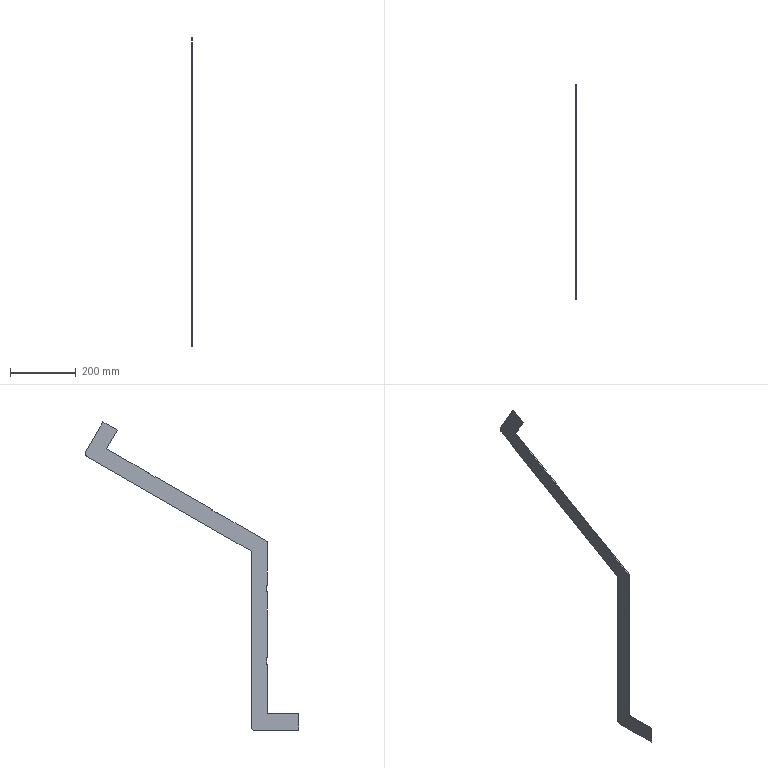Part | STEP file | zzh002 | 1 solid | 30 faces | box 3 x 648.349 x 935.758 mm | volume 197054 mm3 | plane 28 | cylinder 2 | commonest cylinder face diameters 20 x2
STEP:
#1=CARTESIAN_POINT('',(0.,380.183,431.016));
#2=VERTEX_POINT('',#1);
#3=CARTESIAN_POINT('',(0.,379.183,432.748));
#4=VERTEX_POINT('',#3);
#5=CARTESIAN_POINT('',(0.,380.183,431.016));
#6=DIRECTION('',(0.,-0.5,0.866));
#7=VECTOR('',#6,1000.);
#8=LINE('',#5,#7);
#9=EDGE_CURVE('',#2,#4,#8,.T.);
#10=ORIENTED_EDGE('',*,*,#9,.T.);
#11=CARTESIAN_POINT('',(0.,205.978,332.748));
#12=VERTEX_POINT('',#11);
#13=CARTESIAN_POINT('',(0.,379.183,432.748));
#14=DIRECTION('',(0.,-0.866,-0.5));
#15=VECTOR('',#14,1000.);
#16=LINE('',#13,#15);
#17=EDGE_CURVE('',#4,#12,#16,.T.);
#18=ORIENTED_EDGE('',*,*,#17,.T.);
#19=CARTESIAN_POINT('',(0.,206.978,331.016));
#20=VERTEX_POINT('',#19);
#21=CARTESIAN_POINT('',(0.,205.978,332.748));
#22=DIRECTION('',(0.,0.5,-0.866));
#23=VECTOR('',#22,1000.);
#24=LINE('',#21,#23);
#25=EDGE_CURVE('',#12,#20,#24,.T.);
#26=ORIENTED_EDGE('',*,*,#25,.T.);
#27=CARTESIAN_POINT('',(0.,189.658,321.016));
#28=VERTEX_POINT('',#27);
#29=CARTESIAN_POINT('',(0.,206.978,331.016));
#30=DIRECTION('',(0.,-0.866,-0.5));
#31=VECTOR('',#30,1000.);
#32=LINE('',#29,#31);
#33=EDGE_CURVE('',#20,#28,#32,.T.);
#34=ORIENTED_EDGE('',*,*,#33,.T.);
#35=CARTESIAN_POINT('',(0.,188.658,322.748));
#36=VERTEX_POINT('',#35);
#37=CARTESIAN_POINT('',(0.,189.658,321.016));
#38=DIRECTION('',(0.,-0.5,0.866));
#39=VECTOR('',#38,1000.);
#40=LINE('',#37,#39);
#41=EDGE_CURVE('',#28,#36,#40,.T.);
#42=ORIENTED_EDGE('',*,*,#41,.T.);
#43=CARTESIAN_POINT('',(0.,37.7,235.592));
#44=VERTEX_POINT('',#43);
#45=CARTESIAN_POINT('',(0.,188.658,322.748));
#46=DIRECTION('',(0.,-0.866,-0.5));
#47=VECTOR('',#46,1000.);
#48=LINE('',#45,#47);
#49=EDGE_CURVE('',#36,#44,#48,.T.);
#50=ORIENTED_EDGE('',*,*,#49,.T.);
#51=CARTESIAN_POINT('',(0.,37.7,103.281));
#52=VERTEX_POINT('',#51);
#53=CARTESIAN_POINT('',(0.,37.7,503.107));
#54=DIRECTION('',(0.,0.,-1.));
#55=VECTOR('',#54,1000.);
#56=LINE('',#53,#55);
#57=EDGE_CURVE('',#44,#52,#56,.T.);
#58=ORIENTED_EDGE('',*,*,#57,.T.);
#59=CARTESIAN_POINT('',(0.,39.7,103.281));
#60=VERTEX_POINT('',#59);
#61=CARTESIAN_POINT('',(0.,581.049,103.281));
#62=DIRECTION('',(0.,1.,0.));
#63=VECTOR('',#62,1000.);
#64=LINE('',#61,#63);
#65=EDGE_CURVE('',#52,#60,#64,.T.);
#66=ORIENTED_EDGE('',*,*,#65,.T.);
#67=CARTESIAN_POINT('',(0.,39.7,83.281));
#68=VERTEX_POINT('',#67);
#69=CARTESIAN_POINT('',(0.,39.7,503.107));
#70=DIRECTION('',(0.,0.,-1.));
#71=VECTOR('',#70,1000.);
#72=LINE('',#69,#71);
#73=EDGE_CURVE('',#60,#68,#72,.T.);
#74=ORIENTED_EDGE('',*,*,#73,.T.);
#75=CARTESIAN_POINT('',(0.,37.7,83.281));
#76=VERTEX_POINT('',#75);
#77=CARTESIAN_POINT('',(0.,581.049,83.281));
#78=DIRECTION('',(0.,-1.,0.));
#79=VECTOR('',#78,1000.);
#80=LINE('',#77,#79);
#81=EDGE_CURVE('',#68,#76,#80,.T.);
#82=ORIENTED_EDGE('',*,*,#81,.T.);
#83=CARTESIAN_POINT('',(0.,37.7,-116.719));
#84=VERTEX_POINT('',#83);
#85=CARTESIAN_POINT('',(0.,37.7,503.107));
#86=DIRECTION('',(0.,0.,-1.));
#87=VECTOR('',#86,1000.);
#88=LINE('',#85,#87);
#89=EDGE_CURVE('',#76,#84,#88,.T.);
#90=ORIENTED_EDGE('',*,*,#89,.T.);
#91=CARTESIAN_POINT('',(0.,39.7,-116.719));
#92=VERTEX_POINT('',#91);
#93=CARTESIAN_POINT('',(0.,581.049,-116.719));
#94=DIRECTION('',(0.,1.,0.));
#95=VECTOR('',#94,1000.);
#96=LINE('',#93,#95);
#97=EDGE_CURVE('',#84,#92,#96,.T.);
#98=ORIENTED_EDGE('',*,*,#97,.T.);
#99=CARTESIAN_POINT('',(0.,39.7,-136.719));
#100=VERTEX_POINT('',#99);
#101=CARTESIAN_POINT('',(0.,39.7,503.107));
#102=DIRECTION('',(0.,0.,-1.));
#103=VECTOR('',#102,1000.);
#104=LINE('',#101,#103);
#105=EDGE_CURVE('',#92,#100,#104,.T.);
#106=ORIENTED_EDGE('',*,*,#105,.T.);
#107=CARTESIAN_POINT('',(0.,37.7,-136.719));
#108=VERTEX_POINT('',#107);
#109=CARTESIAN_POINT('',(0.,581.049,-136.719));
#110=DIRECTION('',(0.,-1.,0.));
#111=VECTOR('',#110,1000.);
#112=LINE('',#109,#111);
#113=EDGE_CURVE('',#100,#108,#112,.T.);
#114=ORIENTED_EDGE('',*,*,#113,.T.);
#115=CARTESIAN_POINT('',(0.,37.7,-286.719));
#116=VERTEX_POINT('',#115);
#117=CARTESIAN_POINT('',(0.,37.7,503.107));
#118=DIRECTION('',(0.,0.,-1.));
#119=VECTOR('',#118,1000.);
#120=LINE('',#117,#119);
#121=EDGE_CURVE('',#108,#116,#120,.T.);
#122=ORIENTED_EDGE('',*,*,#121,.T.);
#123=CARTESIAN_POINT('',(0.,-57.3,-286.719));
#124=VERTEX_POINT('',#123);
#125=CARTESIAN_POINT('',(0.,581.049,-286.719));
#126=DIRECTION('',(0.,-1.,0.));
#127=VECTOR('',#126,1000.);
#128=LINE('',#125,#127);
#129=EDGE_CURVE('',#116,#124,#128,.T.);
#130=ORIENTED_EDGE('',*,*,#129,.T.);
#131=CARTESIAN_POINT('',(0.,-57.3,-336.719));
#132=VERTEX_POINT('',#131);
#133=CARTESIAN_POINT('',(0.,-57.3,503.107));
#134=DIRECTION('',(0.,0.,-1.));
#135=VECTOR('',#134,1000.);
#136=LINE('',#133,#135);
#137=EDGE_CURVE('',#124,#132,#136,.T.);
#138=ORIENTED_EDGE('',*,*,#137,.T.);
#139=CARTESIAN_POINT('',(0.,77.7,-336.719));
#140=VERTEX_POINT('',#139);
#141=CARTESIAN_POINT('',(0.,581.049,-336.719));
#142=DIRECTION('',(0.,1.,0.));
#143=VECTOR('',#142,1000.);
#144=LINE('',#141,#143);
#145=EDGE_CURVE('',#132,#140,#144,.T.);
#146=ORIENTED_EDGE('',*,*,#145,.T.);
#147=CARTESIAN_POINT('',(0.,87.7,-326.719));
#148=VERTEX_POINT('',#147);
#149=CARTESIAN_POINT('',(0.,77.7,-326.719));
#150=DIRECTION('',(1.,0.,0.));
#151=DIRECTION('',(0.,0.,-1.));
#152=AXIS2_PLACEMENT_3D('',#149,#150,#151);
#153=CIRCLE('',#152,10.);
#154=EDGE_CURVE('',#140,#148,#153,.T.);
#155=ORIENTED_EDGE('',*,*,#154,.T.);
#156=CARTESIAN_POINT('',(0.,87.7,206.725));
#157=VERTEX_POINT('',#156);
#158=CARTESIAN_POINT('',(0.,87.7,503.107));
#159=DIRECTION('',(0.,0.,1.));
#160=VECTOR('',#159,1000.);
#161=LINE('',#158,#160);
#162=EDGE_CURVE('',#148,#157,#161,.T.);
#163=ORIENTED_EDGE('',*,*,#162,.T.);
#164=CARTESIAN_POINT('',(0.,586.049,494.446));
#165=VERTEX_POINT('',#164);
#166=CARTESIAN_POINT('',(0.,87.7,206.725));
#167=DIRECTION('',(0.,0.866,0.5));
#168=VECTOR('',#167,1000.);
#169=LINE('',#166,#168);
#170=EDGE_CURVE('',#157,#165,#169,.T.);
#171=ORIENTED_EDGE('',*,*,#170,.T.);
#172=CARTESIAN_POINT('',(0.,589.709,508.107));
#173=VERTEX_POINT('',#172);
#174=CARTESIAN_POINT('',(0.,581.049,503.107));
#175=DIRECTION('',(1.,0.,0.));
#176=DIRECTION('',(0.,0.,-1.));
#177=AXIS2_PLACEMENT_3D('',#174,#175,#176);
#178=CIRCLE('',#177,10.);
#179=EDGE_CURVE('',#165,#173,#178,.T.);
#180=ORIENTED_EDGE('',*,*,#179,.T.);
#181=CARTESIAN_POINT('',(0.,537.209,599.039));
#182=VERTEX_POINT('',#181);
#183=CARTESIAN_POINT('',(0.,589.709,508.107));
#184=DIRECTION('',(0.,-0.5,0.866));
#185=VECTOR('',#184,1000.);
#186=LINE('',#183,#185);
#187=EDGE_CURVE('',#173,#182,#186,.T.);
#188=ORIENTED_EDGE('',*,*,#187,.T.);
#189=CARTESIAN_POINT('',(0.,493.908,574.039));
#190=VERTEX_POINT('',#189);
#191=CARTESIAN_POINT('',(0.,537.209,599.039));
#192=DIRECTION('',(0.,-0.866,-0.5));
#193=VECTOR('',#192,1000.);
#194=LINE('',#191,#193);
#195=EDGE_CURVE('',#182,#190,#194,.T.);
#196=ORIENTED_EDGE('',*,*,#195,.T.);
#197=CARTESIAN_POINT('',(0.,526.408,517.748));
#198=VERTEX_POINT('',#197);
#199=CARTESIAN_POINT('',(0.,493.908,574.039));
#200=DIRECTION('',(0.,0.5,-0.866));
#201=VECTOR('',#200,1000.);
#202=LINE('',#199,#201);
#203=EDGE_CURVE('',#190,#198,#202,.T.);
#204=ORIENTED_EDGE('',*,*,#203,.T.);
#205=CARTESIAN_POINT('',(0.,396.504,442.748));
#206=VERTEX_POINT('',#205);
#207=CARTESIAN_POINT('',(0.,526.408,517.748));
#208=DIRECTION('',(0.,-0.866,-0.5));
#209=VECTOR('',#208,1000.);
#210=LINE('',#207,#209);
#211=EDGE_CURVE('',#198,#206,#210,.T.);
#212=ORIENTED_EDGE('',*,*,#211,.T.);
#213=CARTESIAN_POINT('',(0.,397.504,441.016));
#214=VERTEX_POINT('',#213);
#215=CARTESIAN_POINT('',(0.,396.504,442.748));
#216=DIRECTION('',(0.,0.5,-0.866));
#217=VECTOR('',#216,1000.);
#218=LINE('',#215,#217);
#219=EDGE_CURVE('',#206,#214,#218,.T.);
#220=ORIENTED_EDGE('',*,*,#219,.T.);
#221=CARTESIAN_POINT('',(0.,397.504,441.016));
#222=DIRECTION('',(0.,-0.866,-0.5));
#223=VECTOR('',#222,1000.);
#224=LINE('',#221,#223);
#225=EDGE_CURVE('',#214,#2,#224,.T.);
#226=ORIENTED_EDGE('',*,*,#225,.T.);
#227=EDGE_LOOP('',(#10,#18,#26,#34,#42,#50,#58,#66,#74,#82,#90,#98,#106,#114,#122,#130,#138,#146,#155,#163,#171,#180,#188,#196,#204,#212,#220,#226));
#228=FACE_OUTER_BOUND('',#227,.T.);
#229=CARTESIAN_POINT('',(0.,581.049,503.107));
#230=DIRECTION('',(1.,0.,0.));
#231=DIRECTION('',(0.,0.,-1.));
#232=AXIS2_PLACEMENT_3D('',#229,#230,#231);
#233=PLANE('',#232);
#234=ADVANCED_FACE('',(#228),#233,.T.);
#235=CARTESIAN_POINT('',(-3.,379.183,432.748));
#236=VERTEX_POINT('',#235);
#237=CARTESIAN_POINT('',(-3.,379.183,432.748));
#238=DIRECTION('',(-1.,0.,0.));
#239=VECTOR('',#238,1000.);
#240=LINE('',#237,#239);
#241=EDGE_CURVE('',#4,#236,#240,.T.);
#242=ORIENTED_EDGE('',*,*,#241,.T.);
#243=CARTESIAN_POINT('',(-3.,205.978,332.748));
#244=VERTEX_POINT('',#243);
#245=CARTESIAN_POINT('',(-3.,37.7,235.592));
#246=DIRECTION('',(0.,-0.866,-0.5));
#247=VECTOR('',#246,1000.);
#248=LINE('',#245,#247);
#249=EDGE_CURVE('',#236,#244,#248,.T.);
#250=ORIENTED_EDGE('',*,*,#249,.T.);
#251=CARTESIAN_POINT('',(-3.,205.978,332.748));
#252=DIRECTION('',(1.,0.,0.));
#253=VECTOR('',#252,1000.);
#254=LINE('',#251,#253);
#255=EDGE_CURVE('',#244,#12,#254,.T.);
#256=ORIENTED_EDGE('',*,*,#255,.T.);
#257=ORIENTED_EDGE('',*,*,#17,.F.);
#258=EDGE_LOOP('',(#242,#250,#256,#257));
#259=FACE_OUTER_BOUND('',#258,.T.);
#260=CARTESIAN_POINT('',(-3.,37.7,235.592));
#261=DIRECTION('',(0.,-0.5,0.866));
#262=DIRECTION('',(0.,-0.866,-0.5));
#263=AXIS2_PLACEMENT_3D('',#260,#261,#262);
#264=PLANE('',#263);
#265=ADVANCED_FACE('',(#259),#264,.T.);
#266=ORIENTED_EDGE('',*,*,#241,.F.);
#267=ORIENTED_EDGE('',*,*,#9,.F.);
#268=CARTESIAN_POINT('',(-3.,380.183,431.016));
#269=VERTEX_POINT('',#268);
#270=CARTESIAN_POINT('',(0.,380.183,431.016));
#271=DIRECTION('',(1.,0.,0.));
#272=VECTOR('',#271,1000.);
#273=LINE('',#270,#272);
#274=EDGE_CURVE('',#269,#2,#273,.T.);
#275=ORIENTED_EDGE('',*,*,#274,.F.);
#276=CARTESIAN_POINT('',(-3.,379.183,432.748));
#277=DIRECTION('',(0.,0.5,-0.866));
#278=VECTOR('',#277,1000.);
#279=LINE('',#276,#278);
#280=EDGE_CURVE('',#236,#269,#279,.T.);
#281=ORIENTED_EDGE('',*,*,#280,.F.);
#282=EDGE_LOOP('',(#266,#267,#275,#281));
#283=FACE_OUTER_BOUND('',#282,.T.);
#284=CARTESIAN_POINT('',(0.,379.183,432.748));
#285=DIRECTION('',(0.,-0.866,-0.5));
#286=DIRECTION('',(0.,0.5,-0.866));
#287=AXIS2_PLACEMENT_3D('',#284,#285,#286);
#288=PLANE('',#287);
#289=ADVANCED_FACE('',(#283),#288,.F.);
#290=ORIENTED_EDGE('',*,*,#274,.T.);
#291=ORIENTED_EDGE('',*,*,#225,.F.);
#292=CARTESIAN_POINT('',(-3.,397.504,441.016));
#293=VERTEX_POINT('',#292);
#294=CARTESIAN_POINT('',(0.,397.504,441.016));
#295=DIRECTION('',(1.,0.,0.));
#296=VECTOR('',#295,1000.);
#297=LINE('',#294,#296);
#298=EDGE_CURVE('',#293,#214,#297,.T.);
#299=ORIENTED_EDGE('',*,*,#298,.F.);
#300=CARTESIAN_POINT('',(-3.,397.504,441.016));
#301=DIRECTION('',(0.,0.866,0.5));
#302=VECTOR('',#301,1000.);
#303=LINE('',#300,#302);
#304=EDGE_CURVE('',#269,#293,#303,.T.);
#305=ORIENTED_EDGE('',*,*,#304,.F.);
#306=EDGE_LOOP('',(#290,#291,#299,#305));
#307=FACE_OUTER_BOUND('',#306,.T.);
#308=CARTESIAN_POINT('',(0.,397.504,441.016));
#309=DIRECTION('',(0.,0.5,-0.866));
#310=DIRECTION('',(0.,0.866,0.5));
#311=AXIS2_PLACEMENT_3D('',#308,#309,#310);
#312=PLANE('',#311);
#313=ADVANCED_FACE('',(#307),#312,.F.);
#314=ORIENTED_EDGE('',*,*,#298,.T.);
#315=ORIENTED_EDGE('',*,*,#219,.F.);
#316=CARTESIAN_POINT('',(-3.,396.504,442.748));
#317=VERTEX_POINT('',#316);
#318=CARTESIAN_POINT('',(0.,396.504,442.748));
#319=DIRECTION('',(1.,0.,0.));
#320=VECTOR('',#319,1000.);
#321=LINE('',#318,#320);
#322=EDGE_CURVE('',#317,#206,#321,.T.);
#323=ORIENTED_EDGE('',*,*,#322,.F.);
#324=CARTESIAN_POINT('',(-3.,396.504,442.748));
#325=DIRECTION('',(0.,-0.5,0.866));
#326=VECTOR('',#325,1000.);
#327=LINE('',#324,#326);
#328=EDGE_CURVE('',#293,#317,#327,.T.);
#329=ORIENTED_EDGE('',*,*,#328,.F.);
#330=EDGE_LOOP('',(#314,#315,#323,#329));
#331=FACE_OUTER_BOUND('',#330,.T.);
#332=CARTESIAN_POINT('',(0.,396.504,442.748));
#333=DIRECTION('',(0.,0.866,0.5));
#334=DIRECTION('',(0.,-0.5,0.866));
#335=AXIS2_PLACEMENT_3D('',#332,#333,#334);
#336=PLANE('',#335);
#337=ADVANCED_FACE('',(#331),#336,.F.);
#338=CARTESIAN_POINT('',(-3.,526.408,517.748));
#339=VERTEX_POINT('',#338);
#340=CARTESIAN_POINT('',(-3.,526.408,517.748));
#341=DIRECTION('',(-1.,0.,0.));
#342=VECTOR('',#341,1000.);
#343=LINE('',#340,#342);
#344=EDGE_CURVE('',#198,#339,#343,.T.);
#345=ORIENTED_EDGE('',*,*,#344,.T.);
#346=CARTESIAN_POINT('',(-3.,37.7,235.592));
#347=DIRECTION('',(0.,-0.866,-0.5));
#348=VECTOR('',#347,1000.);
#349=LINE('',#346,#348);
#350=EDGE_CURVE('',#339,#317,#349,.T.);
#351=ORIENTED_EDGE('',*,*,#350,.T.);
#352=ORIENTED_EDGE('',*,*,#322,.T.);
#353=ORIENTED_EDGE('',*,*,#211,.F.);
#354=EDGE_LOOP('',(#345,#351,#352,#353));
#355=FACE_OUTER_BOUND('',#354,.T.);
#356=CARTESIAN_POINT('',(-3.,37.7,235.592));
#357=DIRECTION('',(0.,-0.5,0.866));
#358=DIRECTION('',(0.,-0.866,-0.5));
#359=AXIS2_PLACEMENT_3D('',#356,#357,#358);
#360=PLANE('',#359);
#361=ADVANCED_FACE('',(#355),#360,.T.);
#362=CARTESIAN_POINT('',(-3.,493.908,574.039));
#363=VERTEX_POINT('',#362);
#364=CARTESIAN_POINT('',(-3.,526.408,517.748));
#365=DIRECTION('',(0.,0.5,-0.866));
#366=VECTOR('',#365,1000.);
#367=LINE('',#364,#366);
#368=EDGE_CURVE('',#363,#339,#367,.T.);
#369=ORIENTED_EDGE('',*,*,#368,.T.);
#370=ORIENTED_EDGE('',*,*,#344,.F.);
#371=ORIENTED_EDGE('',*,*,#203,.F.);
#372=CARTESIAN_POINT('',(-3.,493.908,574.039));
#373=DIRECTION('',(-1.,0.,0.));
#374=VECTOR('',#373,1000.);
#375=LINE('',#372,#374);
#376=EDGE_CURVE('',#190,#363,#375,.T.);
#377=ORIENTED_EDGE('',*,*,#376,.T.);
#378=EDGE_LOOP('',(#369,#370,#371,#377));
#379=FACE_OUTER_BOUND('',#378,.T.);
#380=CARTESIAN_POINT('',(-3.,526.408,517.748));
#381=DIRECTION('',(0.,-0.866,-0.5));
#382=DIRECTION('',(0.,0.5,-0.866));
#383=AXIS2_PLACEMENT_3D('',#380,#381,#382);
#384=PLANE('',#383);
#385=ADVANCED_FACE('',(#379),#384,.T.);
#386=CARTESIAN_POINT('',(-3.,537.209,599.039));
#387=VERTEX_POINT('',#386);
#388=CARTESIAN_POINT('',(-3.,537.209,599.039));
#389=DIRECTION('',(0.,-0.866,-0.5));
#390=VECTOR('',#389,1000.);
#391=LINE('',#388,#390);
#392=EDGE_CURVE('',#387,#363,#391,.T.);
#393=ORIENTED_EDGE('',*,*,#392,.T.);
#394=ORIENTED_EDGE('',*,*,#376,.F.);
#395=ORIENTED_EDGE('',*,*,#195,.F.);
#396=CARTESIAN_POINT('',(-3.,537.209,599.039));
#397=DIRECTION('',(-1.,0.,0.));
#398=VECTOR('',#397,1000.);
#399=LINE('',#396,#398);
#400=EDGE_CURVE('',#182,#387,#399,.T.);
#401=ORIENTED_EDGE('',*,*,#400,.T.);
#402=EDGE_LOOP('',(#393,#394,#395,#401));
#403=FACE_OUTER_BOUND('',#402,.T.);
#404=CARTESIAN_POINT('',(-3.,537.209,599.039));
#405=DIRECTION('',(0.,-0.5,0.866));
#406=DIRECTION('',(0.,-0.866,-0.5));
#407=AXIS2_PLACEMENT_3D('',#404,#405,#406);
#408=PLANE('',#407);
#409=ADVANCED_FACE('',(#403),#408,.T.);
#410=CARTESIAN_POINT('',(-3.,589.709,508.107));
#411=VERTEX_POINT('',#410);
#412=CARTESIAN_POINT('',(-3.,589.709,508.107));
#413=DIRECTION('',(0.,-0.5,0.866));
#414=VECTOR('',#413,1000.);
#415=LINE('',#412,#414);
#416=EDGE_CURVE('',#411,#387,#415,.T.);
#417=ORIENTED_EDGE('',*,*,#416,.T.);
#418=ORIENTED_EDGE('',*,*,#400,.F.);
#419=ORIENTED_EDGE('',*,*,#187,.F.);
#420=CARTESIAN_POINT('',(-3.,589.709,508.107));
#421=DIRECTION('',(-1.,0.,0.));
#422=VECTOR('',#421,1000.);
#423=LINE('',#420,#422);
#424=EDGE_CURVE('',#173,#411,#423,.T.);
#425=ORIENTED_EDGE('',*,*,#424,.T.);
#426=EDGE_LOOP('',(#417,#418,#419,#425));
#427=FACE_OUTER_BOUND('',#426,.T.);
#428=CARTESIAN_POINT('',(-3.,589.709,508.107));
#429=DIRECTION('',(0.,0.866,0.5));
#430=DIRECTION('',(0.,-0.5,0.866));
#431=AXIS2_PLACEMENT_3D('',#428,#429,#430);
#432=PLANE('',#431);
#433=ADVANCED_FACE('',(#427),#432,.T.);
#434=CARTESIAN_POINT('',(-3.,586.049,494.446));
#435=VERTEX_POINT('',#434);
#436=CARTESIAN_POINT('',(-3.,581.049,503.107));
#437=DIRECTION('',(1.,0.,0.));
#438=DIRECTION('',(0.,0.,-1.));
#439=AXIS2_PLACEMENT_3D('',#436,#437,#438);
#440=CIRCLE('',#439,10.);
#441=EDGE_CURVE('',#435,#411,#440,.T.);
#442=ORIENTED_EDGE('',*,*,#441,.T.);
#443=ORIENTED_EDGE('',*,*,#424,.F.);
#444=ORIENTED_EDGE('',*,*,#179,.F.);
#445=CARTESIAN_POINT('',(-3.,586.049,494.446));
#446=DIRECTION('',(-1.,0.,0.));
#447=VECTOR('',#446,1000.);
#448=LINE('',#445,#447);
#449=EDGE_CURVE('',#165,#435,#448,.T.);
#450=ORIENTED_EDGE('',*,*,#449,.T.);
#451=EDGE_LOOP('',(#442,#443,#444,#450));
#452=FACE_OUTER_BOUND('',#451,.T.);
#453=CARTESIAN_POINT('',(-3.,581.049,503.107));
#454=DIRECTION('',(1.,0.,0.));
#455=DIRECTION('',(0.,0.,-1.));
#456=AXIS2_PLACEMENT_3D('',#453,#454,#455);
#457=CYLINDRICAL_SURFACE('',#456,10.);
#458=ADVANCED_FACE('',(#452),#457,.T.);
#459=CARTESIAN_POINT('',(-3.,87.7,206.725));
#460=VERTEX_POINT('',#459);
#461=CARTESIAN_POINT('',(-3.,87.7,206.725));
#462=DIRECTION('',(0.,0.866,0.5));
#463=VECTOR('',#462,1000.);
#464=LINE('',#461,#463);
#465=EDGE_CURVE('',#460,#435,#464,.T.);
#466=ORIENTED_EDGE('',*,*,#465,.T.);
#467=ORIENTED_EDGE('',*,*,#449,.F.);
#468=ORIENTED_EDGE('',*,*,#170,.F.);
#469=CARTESIAN_POINT('',(-3.,87.7,206.725));
#470=DIRECTION('',(-1.,0.,0.));
#471=VECTOR('',#470,1000.);
#472=LINE('',#469,#471);
#473=EDGE_CURVE('',#157,#460,#472,.T.);
#474=ORIENTED_EDGE('',*,*,#473,.T.);
#475=EDGE_LOOP('',(#466,#467,#468,#474));
#476=FACE_OUTER_BOUND('',#475,.T.);
#477=CARTESIAN_POINT('',(-3.,87.7,206.725));
#478=DIRECTION('',(0.,0.5,-0.866));
#479=DIRECTION('',(0.,0.866,0.5));
#480=AXIS2_PLACEMENT_3D('',#477,#478,#479);
#481=PLANE('',#480);
#482=ADVANCED_FACE('',(#476),#481,.T.);
#483=CARTESIAN_POINT('',(-3.,87.7,-326.719));
#484=VERTEX_POINT('',#483);
#485=CARTESIAN_POINT('',(-3.,87.7,-326.719));
#486=DIRECTION('',(0.,0.,1.));
#487=VECTOR('',#486,1000.);
#488=LINE('',#485,#487);
#489=EDGE_CURVE('',#484,#460,#488,.T.);
#490=ORIENTED_EDGE('',*,*,#489,.T.);
#491=ORIENTED_EDGE('',*,*,#473,.F.);
#492=ORIENTED_EDGE('',*,*,#162,.F.);
#493=CARTESIAN_POINT('',(-3.,87.7,-326.719));
#494=DIRECTION('',(-1.,0.,0.));
#495=VECTOR('',#494,1000.);
#496=LINE('',#493,#495);
#497=EDGE_CURVE('',#148,#484,#496,.T.);
#498=ORIENTED_EDGE('',*,*,#497,.T.);
#499=EDGE_LOOP('',(#490,#491,#492,#498));
#500=FACE_OUTER_BOUND('',#499,.T.);
#501=CARTESIAN_POINT('',(-3.,87.7,-326.719));
#502=DIRECTION('',(0.,1.,0.));
#503=DIRECTION('',(0.,0.,1.));
#504=AXIS2_PLACEMENT_3D('',#501,#502,#503);
#505=PLANE('',#504);
#506=ADVANCED_FACE('',(#500),#505,.T.);
#507=CARTESIAN_POINT('',(-3.,77.7,-336.719));
#508=VERTEX_POINT('',#507);
#509=CARTESIAN_POINT('',(-3.,77.7,-326.719));
#510=DIRECTION('',(1.,0.,0.));
#511=DIRECTION('',(0.,0.,-1.));
#512=AXIS2_PLACEMENT_3D('',#509,#510,#511);
#513=CIRCLE('',#512,10.);
#514=EDGE_CURVE('',#508,#484,#513,.T.);
#515=ORIENTED_EDGE('',*,*,#514,.T.);
#516=ORIENTED_EDGE('',*,*,#497,.F.);
#517=ORIENTED_EDGE('',*,*,#154,.F.);
#518=CARTESIAN_POINT('',(-3.,77.7,-336.719));
#519=DIRECTION('',(-1.,0.,0.));
#520=VECTOR('',#519,1000.);
#521=LINE('',#518,#520);
#522=EDGE_CURVE('',#140,#508,#521,.T.);
#523=ORIENTED_EDGE('',*,*,#522,.T.);
#524=EDGE_LOOP('',(#515,#516,#517,#523));
#525=FACE_OUTER_BOUND('',#524,.T.);
#526=CARTESIAN_POINT('',(-3.,77.7,-326.719));
#527=DIRECTION('',(1.,0.,0.));
#528=DIRECTION('',(0.,0.,-1.));
#529=AXIS2_PLACEMENT_3D('',#526,#527,#528);
#530=CYLINDRICAL_SURFACE('',#529,10.);
#531=ADVANCED_FACE('',(#525),#530,.T.);
#532=CARTESIAN_POINT('',(-3.,-57.3,-336.719));
#533=VERTEX_POINT('',#532);
#534=CARTESIAN_POINT('',(-3.,-52.5,-336.719));
#535=DIRECTION('',(0.,1.,0.));
#536=VECTOR('',#535,1000.);
#537=LINE('',#534,#536);
#538=EDGE_CURVE('',#533,#508,#537,.T.);
#539=ORIENTED_EDGE('',*,*,#538,.T.);
#540=ORIENTED_EDGE('',*,*,#522,.F.);
#541=ORIENTED_EDGE('',*,*,#145,.F.);
#542=CARTESIAN_POINT('',(-3.,-57.3,-336.719));
#543=DIRECTION('',(-1.,0.,0.));
#544=VECTOR('',#543,1000.);
#545=LINE('',#542,#544);
#546=EDGE_CURVE('',#132,#533,#545,.T.);
#547=ORIENTED_EDGE('',*,*,#546,.T.);
#548=EDGE_LOOP('',(#539,#540,#541,#547));
#549=FACE_OUTER_BOUND('',#548,.T.);
#550=CARTESIAN_POINT('',(-3.,-52.5,-336.719));
#551=DIRECTION('',(0.,0.,-1.));
#552=DIRECTION('',(0.,1.,0.));
#553=AXIS2_PLACEMENT_3D('',#550,#551,#552);
#554=PLANE('',#553);
#555=ADVANCED_FACE('',(#549),#554,.T.);
#556=CARTESIAN_POINT('',(-3.,-57.3,-286.719));
#557=VERTEX_POINT('',#556);
#558=CARTESIAN_POINT('',(-3.,-57.3,-286.719));
#559=DIRECTION('',(0.,0.,-1.));
#560=VECTOR('',#559,1000.);
#561=LINE('',#558,#560);
#562=EDGE_CURVE('',#557,#533,#561,.T.);
#563=ORIENTED_EDGE('',*,*,#562,.T.);
#564=ORIENTED_EDGE('',*,*,#546,.F.);
#565=ORIENTED_EDGE('',*,*,#137,.F.);
#566=CARTESIAN_POINT('',(-3.,-57.3,-286.719));
#567=DIRECTION('',(-1.,0.,0.));
#568=VECTOR('',#567,1000.);
#569=LINE('',#566,#568);
#570=EDGE_CURVE('',#124,#557,#569,.T.);
#571=ORIENTED_EDGE('',*,*,#570,.T.);
#572=EDGE_LOOP('',(#563,#564,#565,#571));
#573=FACE_OUTER_BOUND('',#572,.T.);
#574=CARTESIAN_POINT('',(-3.,-57.3,-286.719));
#575=DIRECTION('',(0.,-1.,0.));
#576=DIRECTION('',(0.,0.,-1.));
#577=AXIS2_PLACEMENT_3D('',#574,#575,#576);
#578=PLANE('',#577);
#579=ADVANCED_FACE('',(#573),#578,.T.);
#580=CARTESIAN_POINT('',(-3.,37.7,-286.719));
#581=VERTEX_POINT('',#580);
#582=CARTESIAN_POINT('',(-3.,-52.5,-286.719));
#583=DIRECTION('',(0.,-1.,0.));
#584=VECTOR('',#583,1000.);
#585=LINE('',#582,#584);
#586=EDGE_CURVE('',#581,#557,#585,.T.);
#587=ORIENTED_EDGE('',*,*,#586,.T.);
#588=ORIENTED_EDGE('',*,*,#570,.F.);
#589=ORIENTED_EDGE('',*,*,#129,.F.);
#590=CARTESIAN_POINT('',(-3.,37.7,-286.719));
#591=DIRECTION('',(-1.,0.,0.));
#592=VECTOR('',#591,1000.);
#593=LINE('',#590,#592);
#594=EDGE_CURVE('',#116,#581,#593,.T.);
#595=ORIENTED_EDGE('',*,*,#594,.T.);
#596=EDGE_LOOP('',(#587,#588,#589,#595));
#597=FACE_OUTER_BOUND('',#596,.T.);
#598=CARTESIAN_POINT('',(-3.,-52.5,-286.719));
#599=DIRECTION('',(0.,0.,1.));
#600=DIRECTION('',(1.,0.,0.));
#601=AXIS2_PLACEMENT_3D('',#598,#599,#600);
#602=PLANE('',#601);
#603=ADVANCED_FACE('',(#597),#602,.T.);
#604=ORIENTED_EDGE('',*,*,#594,.F.);
#605=ORIENTED_EDGE('',*,*,#121,.F.);
#606=CARTESIAN_POINT('',(-3.,37.7,-136.719));
#607=VERTEX_POINT('',#606);
#608=CARTESIAN_POINT('',(-3.,37.7,-136.719));
#609=DIRECTION('',(-1.,0.,0.));
#610=VECTOR('',#609,1000.);
#611=LINE('',#608,#610);
#612=EDGE_CURVE('',#108,#607,#611,.T.);
#613=ORIENTED_EDGE('',*,*,#612,.T.);
#614=CARTESIAN_POINT('',(-3.,37.7,-286.719));
#615=DIRECTION('',(0.,0.,-1.));
#616=VECTOR('',#615,1000.);
#617=LINE('',#614,#616);
#618=EDGE_CURVE('',#607,#581,#617,.T.);
#619=ORIENTED_EDGE('',*,*,#618,.T.);
#620=EDGE_LOOP('',(#604,#605,#613,#619));
#621=FACE_OUTER_BOUND('',#620,.T.);
#622=CARTESIAN_POINT('',(-3.,37.7,-286.719));
#623=DIRECTION('',(0.,-1.,0.));
#624=DIRECTION('',(0.,0.,-1.));
#625=AXIS2_PLACEMENT_3D('',#622,#623,#624);
#626=PLANE('',#625);
#627=ADVANCED_FACE('',(#621),#626,.T.);
#628=ORIENTED_EDGE('',*,*,#612,.F.);
#629=ORIENTED_EDGE('',*,*,#113,.F.);
#630=CARTESIAN_POINT('',(-3.,39.7,-136.719));
#631=VERTEX_POINT('',#630);
#632=CARTESIAN_POINT('',(0.,39.7,-136.719));
#633=DIRECTION('',(1.,0.,0.));
#634=VECTOR('',#633,1000.);
#635=LINE('',#632,#634);
#636=EDGE_CURVE('',#631,#100,#635,.T.);
#637=ORIENTED_EDGE('',*,*,#636,.F.);
#638=CARTESIAN_POINT('',(-3.,37.7,-136.719));
#639=DIRECTION('',(0.,1.,0.));
#640=VECTOR('',#639,1000.);
#641=LINE('',#638,#640);
#642=EDGE_CURVE('',#607,#631,#641,.T.);
#643=ORIENTED_EDGE('',*,*,#642,.F.);
#644=EDGE_LOOP('',(#628,#629,#637,#643));
#645=FACE_OUTER_BOUND('',#644,.T.);
#646=CARTESIAN_POINT('',(0.,37.7,-136.719));
#647=DIRECTION('',(0.,0.,-1.));
#648=DIRECTION('',(-1.,0.,0.));
#649=AXIS2_PLACEMENT_3D('',#646,#647,#648);
#650=PLANE('',#649);
#651=ADVANCED_FACE('',(#645),#650,.F.);
#652=ORIENTED_EDGE('',*,*,#636,.T.);
#653=ORIENTED_EDGE('',*,*,#105,.F.);
#654=CARTESIAN_POINT('',(-3.,39.7,-116.719));
#655=VERTEX_POINT('',#654);
#656=CARTESIAN_POINT('',(0.,39.7,-116.719));
#657=DIRECTION('',(1.,0.,0.));
#658=VECTOR('',#657,1000.);
#659=LINE('',#656,#658);
#660=EDGE_CURVE('',#655,#92,#659,.T.);
#661=ORIENTED_EDGE('',*,*,#660,.F.);
#662=CARTESIAN_POINT('',(-3.,39.7,-136.719));
#663=DIRECTION('',(0.,0.,1.));
#664=VECTOR('',#663,1000.);
#665=LINE('',#662,#664);
#666=EDGE_CURVE('',#631,#655,#665,.T.);
#667=ORIENTED_EDGE('',*,*,#666,.F.);
#668=EDGE_LOOP('',(#652,#653,#661,#667));
#669=FACE_OUTER_BOUND('',#668,.T.);
#670=CARTESIAN_POINT('',(0.,39.7,-136.719));
#671=DIRECTION('',(0.,1.,0.));
#672=DIRECTION('',(0.,0.,1.));
#673=AXIS2_PLACEMENT_3D('',#670,#671,#672);
#674=PLANE('',#673);
#675=ADVANCED_FACE('',(#669),#674,.F.);
#676=ORIENTED_EDGE('',*,*,#660,.T.);
#677=ORIENTED_EDGE('',*,*,#97,.F.);
#678=CARTESIAN_POINT('',(-3.,37.7,-116.719));
#679=VERTEX_POINT('',#678);
#680=CARTESIAN_POINT('',(0.,37.7,-116.719));
#681=DIRECTION('',(1.,0.,0.));
#682=VECTOR('',#681,1000.);
#683=LINE('',#680,#682);
#684=EDGE_CURVE('',#679,#84,#683,.T.);
#685=ORIENTED_EDGE('',*,*,#684,.F.);
#686=CARTESIAN_POINT('',(-3.,37.7,-116.719));
#687=DIRECTION('',(0.,-1.,0.));
#688=VECTOR('',#687,1000.);
#689=LINE('',#686,#688);
#690=EDGE_CURVE('',#655,#679,#689,.T.);
#691=ORIENTED_EDGE('',*,*,#690,.F.);
#692=EDGE_LOOP('',(#676,#677,#685,#691));
#693=FACE_OUTER_BOUND('',#692,.T.);
#694=CARTESIAN_POINT('',(0.,37.7,-116.719));
#695=DIRECTION('',(0.,0.,1.));
#696=DIRECTION('',(1.,0.,0.));
#697=AXIS2_PLACEMENT_3D('',#694,#695,#696);
#698=PLANE('',#697);
#699=ADVANCED_FACE('',(#693),#698,.F.);
#700=ORIENTED_EDGE('',*,*,#684,.T.);
#701=ORIENTED_EDGE('',*,*,#89,.F.);
#702=CARTESIAN_POINT('',(-3.,37.7,83.281));
#703=VERTEX_POINT('',#702);
#704=CARTESIAN_POINT('',(-3.,37.7,83.281));
#705=DIRECTION('',(-1.,0.,0.));
#706=VECTOR('',#705,1000.);
#707=LINE('',#704,#706);
#708=EDGE_CURVE('',#76,#703,#707,.T.);
#709=ORIENTED_EDGE('',*,*,#708,.T.);
#710=CARTESIAN_POINT('',(-3.,37.7,-286.719));
#711=DIRECTION('',(0.,0.,-1.));
#712=VECTOR('',#711,1000.);
#713=LINE('',#710,#712);
#714=EDGE_CURVE('',#703,#679,#713,.T.);
#715=ORIENTED_EDGE('',*,*,#714,.T.);
#716=EDGE_LOOP('',(#700,#701,#709,#715));
#717=FACE_OUTER_BOUND('',#716,.T.);
#718=CARTESIAN_POINT('',(-3.,37.7,-286.719));
#719=DIRECTION('',(0.,-1.,0.));
#720=DIRECTION('',(0.,0.,-1.));
#721=AXIS2_PLACEMENT_3D('',#718,#719,#720);
#722=PLANE('',#721);
#723=ADVANCED_FACE('',(#717),#722,.T.);
#724=ORIENTED_EDGE('',*,*,#708,.F.);
#725=ORIENTED_EDGE('',*,*,#81,.F.);
#726=CARTESIAN_POINT('',(-3.,39.7,83.281));
#727=VERTEX_POINT('',#726);
#728=CARTESIAN_POINT('',(0.,39.7,83.281));
#729=DIRECTION('',(1.,0.,0.));
#730=VECTOR('',#729,1000.);
#731=LINE('',#728,#730);
#732=EDGE_CURVE('',#727,#68,#731,.T.);
#733=ORIENTED_EDGE('',*,*,#732,.F.);
#734=CARTESIAN_POINT('',(-3.,37.7,83.281));
#735=DIRECTION('',(0.,1.,0.));
#736=VECTOR('',#735,1000.);
#737=LINE('',#734,#736);
#738=EDGE_CURVE('',#703,#727,#737,.T.);
#739=ORIENTED_EDGE('',*,*,#738,.F.);
#740=EDGE_LOOP('',(#724,#725,#733,#739));
#741=FACE_OUTER_BOUND('',#740,.T.);
#742=CARTESIAN_POINT('',(0.,37.7,83.281));
#743=DIRECTION('',(0.,0.,-1.));
#744=DIRECTION('',(-1.,0.,0.));
#745=AXIS2_PLACEMENT_3D('',#742,#743,#744);
#746=PLANE('',#745);
#747=ADVANCED_FACE('',(#741),#746,.F.);
#748=ORIENTED_EDGE('',*,*,#732,.T.);
#749=ORIENTED_EDGE('',*,*,#73,.F.);
#750=CARTESIAN_POINT('',(-3.,39.7,103.281));
#751=VERTEX_POINT('',#750);
#752=CARTESIAN_POINT('',(0.,39.7,103.281));
#753=DIRECTION('',(1.,0.,0.));
#754=VECTOR('',#753,1000.);
#755=LINE('',#752,#754);
#756=EDGE_CURVE('',#751,#60,#755,.T.);
#757=ORIENTED_EDGE('',*,*,#756,.F.);
#758=CARTESIAN_POINT('',(-3.,39.7,83.281));
#759=DIRECTION('',(0.,0.,1.));
#760=VECTOR('',#759,1000.);
#761=LINE('',#758,#760);
#762=EDGE_CURVE('',#727,#751,#761,.T.);
#763=ORIENTED_EDGE('',*,*,#762,.F.);
#764=EDGE_LOOP('',(#748,#749,#757,#763));
#765=FACE_OUTER_BOUND('',#764,.T.);
#766=CARTESIAN_POINT('',(0.,39.7,83.281));
#767=DIRECTION('',(0.,1.,0.));
#768=DIRECTION('',(0.,0.,1.));
#769=AXIS2_PLACEMENT_3D('',#766,#767,#768);
#770=PLANE('',#769);
#771=ADVANCED_FACE('',(#765),#770,.F.);
#772=ORIENTED_EDGE('',*,*,#756,.T.);
#773=ORIENTED_EDGE('',*,*,#65,.F.);
#774=CARTESIAN_POINT('',(-3.,37.7,103.281));
#775=VERTEX_POINT('',#774);
#776=CARTESIAN_POINT('',(0.,37.7,103.281));
#777=DIRECTION('',(1.,0.,0.));
#778=VECTOR('',#777,1000.);
#779=LINE('',#776,#778);
#780=EDGE_CURVE('',#775,#52,#779,.T.);
#781=ORIENTED_EDGE('',*,*,#780,.F.);
#782=CARTESIAN_POINT('',(-3.,37.7,103.281));
#783=DIRECTION('',(0.,-1.,0.));
#784=VECTOR('',#783,1000.);
#785=LINE('',#782,#784);
#786=EDGE_CURVE('',#751,#775,#785,.T.);
#787=ORIENTED_EDGE('',*,*,#786,.F.);
#788=EDGE_LOOP('',(#772,#773,#781,#787));
#789=FACE_OUTER_BOUND('',#788,.T.);
#790=CARTESIAN_POINT('',(0.,37.7,103.281));
#791=DIRECTION('',(0.,0.,1.));
#792=DIRECTION('',(1.,0.,0.));
#793=AXIS2_PLACEMENT_3D('',#790,#791,#792);
#794=PLANE('',#793);
#795=ADVANCED_FACE('',(#789),#794,.F.);
#796=CARTESIAN_POINT('',(-3.,37.7,235.592));
#797=VERTEX_POINT('',#796);
#798=CARTESIAN_POINT('',(-3.,37.7,235.592));
#799=DIRECTION('',(-1.,0.,0.));
#800=VECTOR('',#799,1000.);
#801=LINE('',#798,#800);
#802=EDGE_CURVE('',#44,#797,#801,.T.);
#803=ORIENTED_EDGE('',*,*,#802,.T.);
#804=CARTESIAN_POINT('',(-3.,37.7,-286.719));
#805=DIRECTION('',(0.,0.,-1.));
#806=VECTOR('',#805,1000.);
#807=LINE('',#804,#806);
#808=EDGE_CURVE('',#797,#775,#807,.T.);
#809=ORIENTED_EDGE('',*,*,#808,.T.);
#810=ORIENTED_EDGE('',*,*,#780,.T.);
#811=ORIENTED_EDGE('',*,*,#57,.F.);
#812=EDGE_LOOP('',(#803,#809,#810,#811));
#813=FACE_OUTER_BOUND('',#812,.T.);
#814=CARTESIAN_POINT('',(-3.,37.7,-286.719));
#815=DIRECTION('',(0.,-1.,0.));
#816=DIRECTION('',(0.,0.,-1.));
#817=AXIS2_PLACEMENT_3D('',#814,#815,#816);
#818=PLANE('',#817);
#819=ADVANCED_FACE('',(#813),#818,.T.);
#820=ORIENTED_EDGE('',*,*,#802,.F.);
#821=ORIENTED_EDGE('',*,*,#49,.F.);
#822=CARTESIAN_POINT('',(-3.,188.658,322.748));
#823=VERTEX_POINT('',#822);
#824=CARTESIAN_POINT('',(-3.,188.658,322.748));
#825=DIRECTION('',(-1.,0.,0.));
#826=VECTOR('',#825,1000.);
#827=LINE('',#824,#826);
#828=EDGE_CURVE('',#36,#823,#827,.T.);
#829=ORIENTED_EDGE('',*,*,#828,.T.);
#830=CARTESIAN_POINT('',(-3.,37.7,235.592));
#831=DIRECTION('',(0.,-0.866,-0.5));
#832=VECTOR('',#831,1000.);
#833=LINE('',#830,#832);
#834=EDGE_CURVE('',#823,#797,#833,.T.);
#835=ORIENTED_EDGE('',*,*,#834,.T.);
#836=EDGE_LOOP('',(#820,#821,#829,#835));
#837=FACE_OUTER_BOUND('',#836,.T.);
#838=CARTESIAN_POINT('',(-3.,37.7,235.592));
#839=DIRECTION('',(0.,-0.5,0.866));
#840=DIRECTION('',(0.,-0.866,-0.5));
#841=AXIS2_PLACEMENT_3D('',#838,#839,#840);
#842=PLANE('',#841);
#843=ADVANCED_FACE('',(#837),#842,.T.);
#844=ORIENTED_EDGE('',*,*,#828,.F.);
#845=ORIENTED_EDGE('',*,*,#41,.F.);
#846=CARTESIAN_POINT('',(-3.,189.658,321.016));
#847=VERTEX_POINT('',#846);
#848=CARTESIAN_POINT('',(0.,189.658,321.016));
#849=DIRECTION('',(1.,0.,0.));
#850=VECTOR('',#849,1000.);
#851=LINE('',#848,#850);
#852=EDGE_CURVE('',#847,#28,#851,.T.);
#853=ORIENTED_EDGE('',*,*,#852,.F.);
#854=CARTESIAN_POINT('',(-3.,188.658,322.748));
#855=DIRECTION('',(0.,0.5,-0.866));
#856=VECTOR('',#855,1000.);
#857=LINE('',#854,#856);
#858=EDGE_CURVE('',#823,#847,#857,.T.);
#859=ORIENTED_EDGE('',*,*,#858,.F.);
#860=EDGE_LOOP('',(#844,#845,#853,#859));
#861=FACE_OUTER_BOUND('',#860,.T.);
#862=CARTESIAN_POINT('',(0.,188.658,322.748));
#863=DIRECTION('',(0.,-0.866,-0.5));
#864=DIRECTION('',(0.,0.5,-0.866));
#865=AXIS2_PLACEMENT_3D('',#862,#863,#864);
#866=PLANE('',#865);
#867=ADVANCED_FACE('',(#861),#866,.F.);
#868=ORIENTED_EDGE('',*,*,#852,.T.);
#869=ORIENTED_EDGE('',*,*,#33,.F.);
#870=CARTESIAN_POINT('',(-3.,206.978,331.016));
#871=VERTEX_POINT('',#870);
#872=CARTESIAN_POINT('',(0.,206.978,331.016));
#873=DIRECTION('',(1.,0.,0.));
#874=VECTOR('',#873,1000.);
#875=LINE('',#872,#874);
#876=EDGE_CURVE('',#871,#20,#875,.T.);
#877=ORIENTED_EDGE('',*,*,#876,.F.);
#878=CARTESIAN_POINT('',(-3.,206.978,331.016));
#879=DIRECTION('',(0.,0.866,0.5));
#880=VECTOR('',#879,1000.);
#881=LINE('',#878,#880);
#882=EDGE_CURVE('',#847,#871,#881,.T.);
#883=ORIENTED_EDGE('',*,*,#882,.F.);
#884=EDGE_LOOP('',(#868,#869,#877,#883));
#885=FACE_OUTER_BOUND('',#884,.T.);
#886=CARTESIAN_POINT('',(0.,206.978,331.016));
#887=DIRECTION('',(0.,0.5,-0.866));
#888=DIRECTION('',(0.,0.866,0.5));
#889=AXIS2_PLACEMENT_3D('',#886,#887,#888);
#890=PLANE('',#889);
#891=ADVANCED_FACE('',(#885),#890,.F.);
#892=ORIENTED_EDGE('',*,*,#876,.T.);
#893=ORIENTED_EDGE('',*,*,#25,.F.);
#894=ORIENTED_EDGE('',*,*,#255,.F.);
#895=CARTESIAN_POINT('',(-3.,205.978,332.748));
#896=DIRECTION('',(0.,-0.5,0.866));
#897=VECTOR('',#896,1000.);
#898=LINE('',#895,#897);
#899=EDGE_CURVE('',#871,#244,#898,.T.);
#900=ORIENTED_EDGE('',*,*,#899,.F.);
#901=EDGE_LOOP('',(#892,#893,#894,#900));
#902=FACE_OUTER_BOUND('',#901,.T.);
#903=CARTESIAN_POINT('',(0.,205.978,332.748));
#904=DIRECTION('',(0.,0.866,0.5));
#905=DIRECTION('',(0.,-0.5,0.866));
#906=AXIS2_PLACEMENT_3D('',#903,#904,#905);
#907=PLANE('',#906);
#908=ADVANCED_FACE('',(#902),#907,.F.);
#909=ORIENTED_EDGE('',*,*,#899,.T.);
#910=ORIENTED_EDGE('',*,*,#249,.F.);
#911=ORIENTED_EDGE('',*,*,#280,.T.);
#912=ORIENTED_EDGE('',*,*,#304,.T.);
#913=ORIENTED_EDGE('',*,*,#328,.T.);
#914=ORIENTED_EDGE('',*,*,#350,.F.);
#915=ORIENTED_EDGE('',*,*,#368,.F.);
#916=ORIENTED_EDGE('',*,*,#392,.F.);
#917=ORIENTED_EDGE('',*,*,#416,.F.);
#918=ORIENTED_EDGE('',*,*,#441,.F.);
#919=ORIENTED_EDGE('',*,*,#465,.F.);
#920=ORIENTED_EDGE('',*,*,#489,.F.);
#921=ORIENTED_EDGE('',*,*,#514,.F.);
#922=ORIENTED_EDGE('',*,*,#538,.F.);
#923=ORIENTED_EDGE('',*,*,#562,.F.);
#924=ORIENTED_EDGE('',*,*,#586,.F.);
#925=ORIENTED_EDGE('',*,*,#618,.F.);
#926=ORIENTED_EDGE('',*,*,#642,.T.);
#927=ORIENTED_EDGE('',*,*,#666,.T.);
#928=ORIENTED_EDGE('',*,*,#690,.T.);
#929=ORIENTED_EDGE('',*,*,#714,.F.);
#930=ORIENTED_EDGE('',*,*,#738,.T.);
#931=ORIENTED_EDGE('',*,*,#762,.T.);
#932=ORIENTED_EDGE('',*,*,#786,.T.);
#933=ORIENTED_EDGE('',*,*,#808,.F.);
#934=ORIENTED_EDGE('',*,*,#834,.F.);
#935=ORIENTED_EDGE('',*,*,#858,.T.);
#936=ORIENTED_EDGE('',*,*,#882,.T.);
#937=EDGE_LOOP('',(#909,#910,#911,#912,#913,#914,#915,#916,#917,#918,#919,#920,#921,#922,#923,#924,#925,#926,#927,#928,#929,#930,#931,#932,#933,#934,#935,#936));
#938=FACE_OUTER_BOUND('',#937,.T.);
#939=CARTESIAN_POINT('',(-3.,581.049,503.107));
#940=DIRECTION('',(1.,0.,0.));
#941=DIRECTION('',(0.,0.,-1.));
#942=AXIS2_PLACEMENT_3D('',#939,#940,#941);
#943=PLANE('',#942);
#944=ADVANCED_FACE('',(#938),#943,.F.);
#945=CLOSED_SHELL('',(#234,#265,#289,#313,#337,#361,#385,#409,#433,#458,#482,#506,#531,#555,#579,#603,#627,#651,#675,#699,#723,#747,#771,#795,#819,#843,#867,#891,#908,#944));
#946=MANIFOLD_SOLID_BREP('',#945);
#947=CARTESIAN_POINT('',(0.,0.,0.));
#948=DIRECTION('',(0.,0.,1.));
#949=DIRECTION('',(1.,0.,0.));
#950=AXIS2_PLACEMENT_3D('',#947,#948,#949);
#951=(LENGTH_UNIT()NAMED_UNIT(*)SI_UNIT(.MILLI.,.METRE.));
#952=UNCERTAINTY_MEASURE_WITH_UNIT(LENGTH_MEASURE(0.00001),#951,'','');
#953=(NAMED_UNIT(*)PLANE_ANGLE_UNIT()SI_UNIT($,.RADIAN.));
#954=(NAMED_UNIT(*)SI_UNIT($,.STERADIAN.)SOLID_ANGLE_UNIT());
#955=(GEOMETRIC_REPRESENTATION_CONTEXT(3)GLOBAL_UNCERTAINTY_ASSIGNED_CONTEXT((#952))GLOBAL_UNIT_ASSIGNED_CONTEXT((#951,#953,#954))REPRESENTATION_CONTEXT('',''));
#956=ADVANCED_BREP_SHAPE_REPRESENTATION('',(#946,#950),#955);